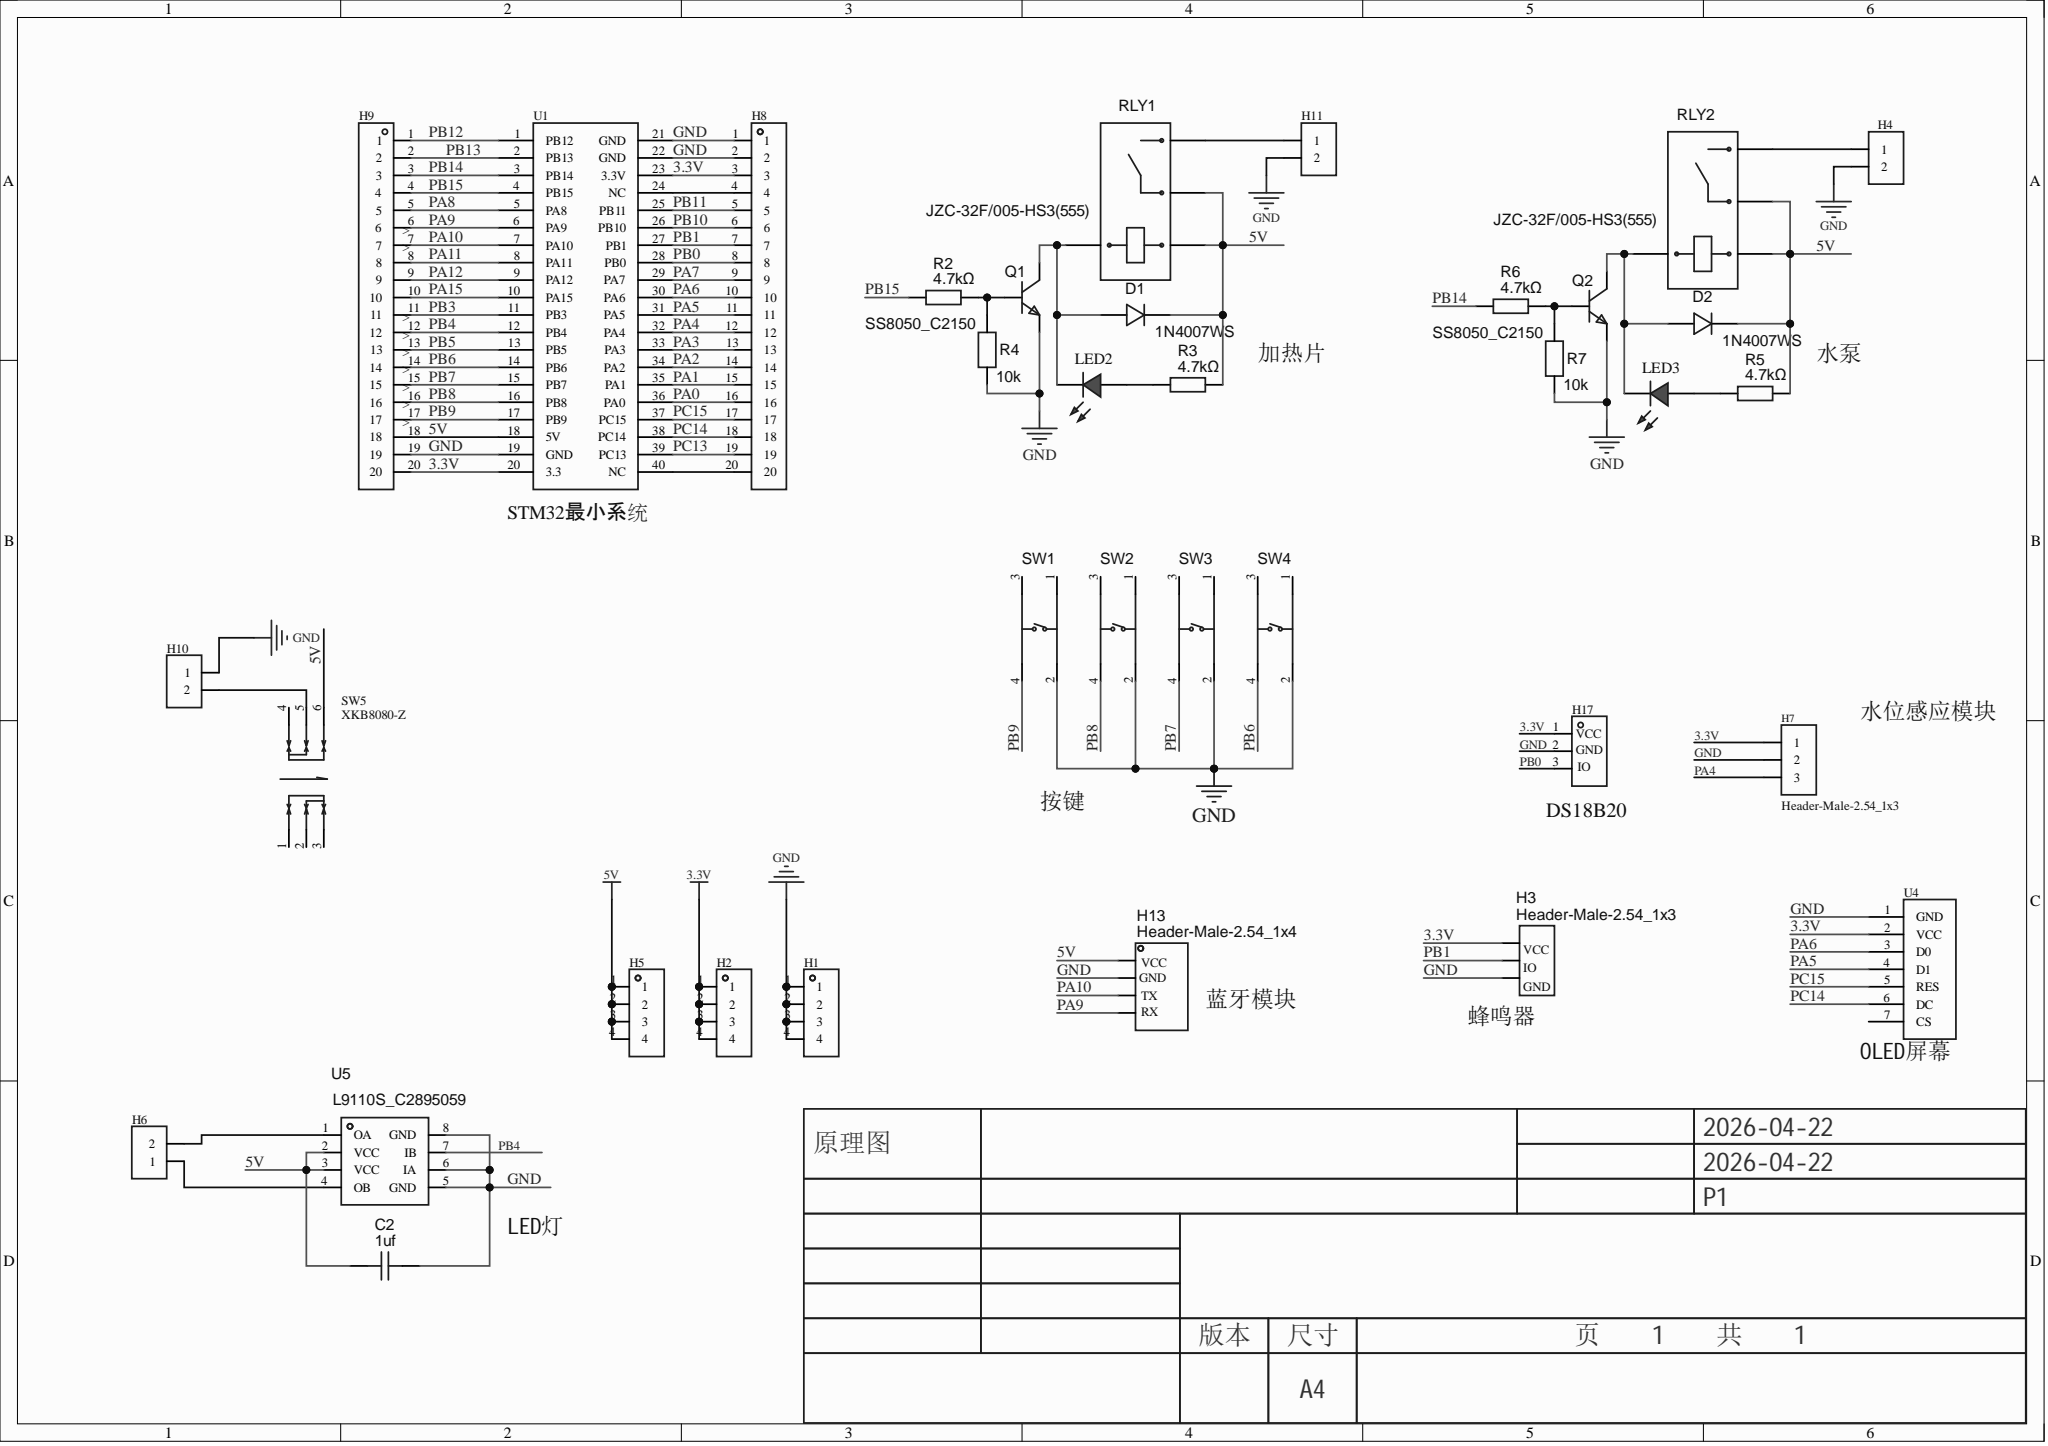Circuit board | Altium Designer | 36 parts | 48 nets
Bill of materials:
Comment,Description,Designator,Footprint,LibRef,Quantity
"1uf","","C2","C0805","1uf","1"
"1N4007WS","","D1, D2","SOD-323_L1.8-W1.3-LS2.5-RD","1N4007WS","2"
"","","H1, H2, H5","HDR-TH_4P-P2.54-V-F","HDR-F_2.54_1x4P","3"
"Header-Male-2.54_1x3","","H3, H7","HDR-TH_3P-P2.54-V-M-1","Header-Male-2.54_1x3","2"
"","","H4, H6, H10, H11","HDR-TH_2P-P2.54-V-F","HDR-F_2.54_1x2P","4"
"","间距:2.54mm;总PIN位数:20;排数:1;插针结构:-;行距:-;安装类型:直插;圆针/方针:-;额定电流:-;额定电压:-;配合针长度:-;塑高:-;触头材质:黄铜;触头镀层:-;颜色:黑色;","H8, H9","HDR-TH_20P-P2.54-V-M-1","HDR-M_2.54_1x20P","2"
"Header-Male-2.54_1x4","","H13","HDR-TH_4P-P2.54-V-M","Header-Male-2.54_1x4","1"
"","","H17","HDR-TH_3P-P2.54-V-F","HDR-F_2.54_1x3P","1"
"","","LED2, LED3","LED_0805","LED_0805-R","2"
"SS8050_C2150","","Q1, Q2","SOT-23-3_L2.9-W1.3-P1.90-LS2.4-BR","SS8050_C2150","2"
"4.7kΩ","","R2, R3, R5, R6","R0805","4.7kΩ","4"
"10k","","R4, R7","R0805","51k","2"
"JZC-32F/005-HS3(555)","","RLY1, RLY2","RELAY-TH_JZC-32F-XXXHXX","JZC-32F/005-HS3(555)","2"
"TS665CJ","","SW1, SW2, SW3, SW4","SW-TH_4P-L6.0-W6.0-P4.50-LS6.5","TS665CJ","4"
"XKB8080-Z","自锁/无锁:自锁;安装方式:直插;触点电流:100mA;额定电压:30V;带灯:不带;作用力:1.6N;工作寿命:10万次;","SW5","SW-TH_6P-L8.0-W8.0-P2.50","XKB8080-Z","1"
"","STM32最小系统","U1","STM32最小系统","STM32最小系统","1"
"","OLED12864/7针","U4","OLED12864/7针","OLED12864/7针","1"
"L9110S_C2895059","","U5","SOP-8_L5.0-W4.0-P1.27-LS6.0-BL","L9110S_C2895059","1"
Netlist (Protel format):
[
C2
C0805
1uf



]
[
D1
SOD-323_L1.8-W1.3-LS2.5-RD
1N4007WS



]
[
D2
SOD-323_L1.8-W1.3-LS2.5-RD
1N4007WS



]
[
H1
HDR-TH_4P-P2.54-V-F




]
[
H2
HDR-TH_4P-P2.54-V-F




]
[
H3
HDR-TH_3P-P2.54-V-M-1
Header-Male-2.54_1x3



]
[
H4
HDR-TH_2P-P2.54-V-F




]
[
H5
HDR-TH_4P-P2.54-V-F




]
[
H6
HDR-TH_2P-P2.54-V-F




]
[
H7
HDR-TH_3P-P2.54-V-M-1
Header-Male-2.54_1x3



]
[
H8
HDR-TH_20P-P2.54-V-M-1




]
[
H9
HDR-TH_20P-P2.54-V-M-1




]
[
H10
HDR-TH_2P-P2.54-V-F




]
[
H11
HDR-TH_2P-P2.54-V-F




]
[
H13
HDR-TH_4P-P2.54-V-M
Header-Male-2.54_1x4



]
[
H17
HDR-TH_3P-P2.54-V-F




]
[
LED2
LED_0805




]
[
LED3
LED_0805




]
[
Q1
SOT-23-3_L2.9-W1.3-P1.90-LS2.4-BR
SS8050_C2150



]
[
Q2
SOT-23-3_L2.9-W1.3-P1.90-LS2.4-BR
SS8050_C2150



]
[
R2
R0805
4.7kΩ



]
[
R3
R0805
4.7kΩ



]
[
R4
R0805
10k



]
[
R5
R0805
4.7kΩ



]
[
R6
R0805
4.7kΩ



]
[
R7
R0805
10k



]
[
RLY1
RELAY-TH_JZC-32F-XXXHXX
JZC-32F/005-HS3(555)



]
[
RLY2
RELAY-TH_JZC-32F-XXXHXX
JZC-32F/005-HS3(555)



]
[
SW1
SW-TH_4P-L6.0-W6.0-P4.50-LS6.5
TS665CJ



]
[
SW2
SW-TH_4P-L6.0-W6.0-P4.50-LS6.5
TS665CJ



]
[
SW3
SW-TH_4P-L6.0-W6.0-P4.50-LS6.5
TS665CJ



]
[
SW4
SW-TH_4P-L6.0-W6.0-P4.50-LS6.5
TS665CJ



]
[
SW5
SW-TH_6P-L8.0-W8.0-P2.50
XKB8080-Z



]
[
U1
STM32最小系统




]
[
U4
OLED12864/7针




]
[
U5
SOP-8_L5.0-W4.0-P1.27-LS6.0-BL
L9110S_C2895059



]
(
PC15
H8-17
U1-37
U4-5
)
(
PC14
H8-18
U1-38
U4-6
)
(
PC13
H8-19
U1-39
)
(
PB15
H9-4
R2-1
U1-4
)
(
PB14
H9-3
R6-1
U1-3
)
(
PB13
H9-2
U1-2
)
(
PB12
H9-1
U1-1
)
(
PB11
H8-5
U1-25
)
(
PB10
H8-6
U1-26
)
(
PB9
H9-17
SW1-4
U1-17
)
(
PB8
H9-16
SW2-4
U1-16
)
(
PB7
H9-15
SW3-4
U1-15
)
(
PB6
H9-14
SW4-4
U1-14
)
(
PB5
H9-13
U1-13
)
(
PB4
H9-12
U1-12
U5-7
)
(
PB3
H9-11
U1-11
)
(
PB1
H3-2
H8-7
U1-27
)
(
PB0
H8-8
H17-3
U1-28
)
(
PA15
H9-10
U1-10
)
(
PA12
H9-9
U1-9
)
(
PA11
H9-8
U1-8
)
(
PA10
H9-7
H13-3
U1-7
)
(
PA9
H9-6
H13-4
U1-6
)
(
PA8
H9-5
U1-5
)
(
PA7
H8-9
U1-29
)
(
PA6
H8-10
U1-30
U4-3
)
(
PA5
H8-11
U1-31
U4-4
)
(
PA4
H7-3
H8-12
U1-32
)
(
PA3
H8-13
U1-33
)
(
PA2
H8-14
U1-34
)
(
PA1
H8-15
U1-35
)
(
PA0
H8-16
U1-36
)
(
NetQ2_1
Q2-1
R6-2
R7-2
)
(
NetQ1_1
Q1-1
R2-2
R4-2
)
(
NetLED3_2
LED3-2
R5-1
)
(
NetLED2_2
LED2-2
R3-1
)
(
NetH11_1
H11-1
RLY1-3
)
(
NetH10_2
H10-2
SW5-5
)
(
NetH8_20
H8-20
U1-40
)
(
NetH8_4
H8-4
U1-24
)
(
NetH6_2
H6-2
U5-1
)
(
NetH6_1
H6-1
U5-4
)
(
NetH4_1
H4-1
RLY2-3
)
(
NetD2_2
D2-2
LED3-1
Q2-3
RLY2-2
)
(
NetD1_2
D1-2
LED2-1
Q1-3
RLY1-2
)
(
GND
C2-2
H1-1
H1-2
H1-3
H1-4
H3-3
H4-2
H7-2
H8-1
H8-2
H9-19
H10-1
H11-2
H13-2
H17-2
Q1-2
Q2-2
R4-1
R7-1
SW1-2
SW2-2
SW3-2
SW4-2
U1-19
U1-21
U1-22
U4-1
U5-5
U5-6
U5-8
)
(
5V
C2-1
D1-1
D2-1
H5-1
H5-2
H5-3
H5-4
H9-18
H13-1
R3-2
R5-2
RLY1-1
RLY1-4
RLY2-1
RLY2-4
SW5-6
U1-18
U5-2
U5-3
)
(
3.3V
H2-1
H2-2
H2-3
H2-4
H3-1
H7-1
H8-3
H9-20
H17-1
U1-20
U1-23
U4-2
)